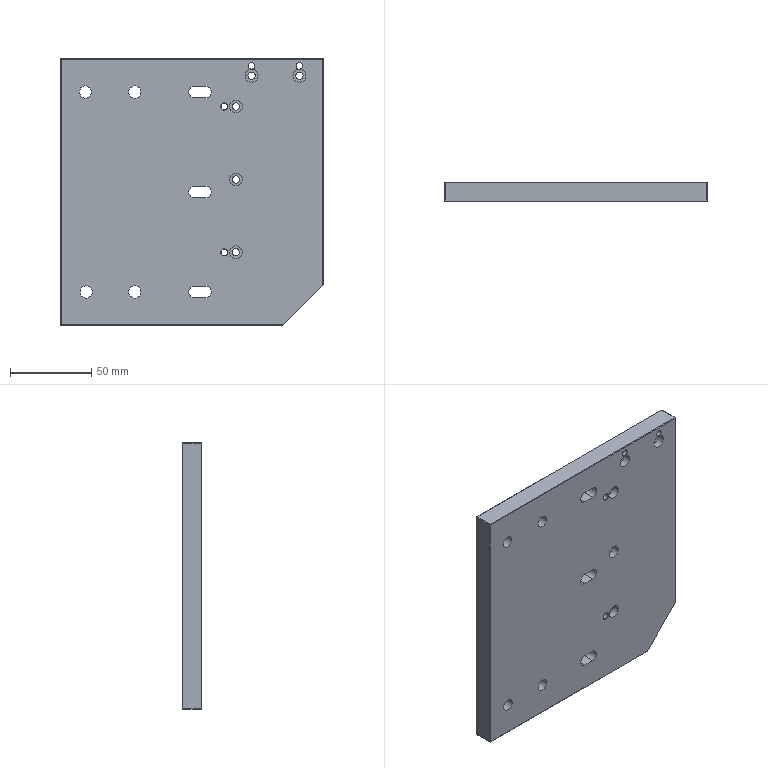Part | NX | 1 solid | 88 faces | box 162 x 12 x 164.5 mm | volume 308404 mm3 | cylinder 45 | plane 31 | cone 12 | commonest cylinder face diameters 4.5 x10 8 x10 7 x9 4 x8 7.5 x8